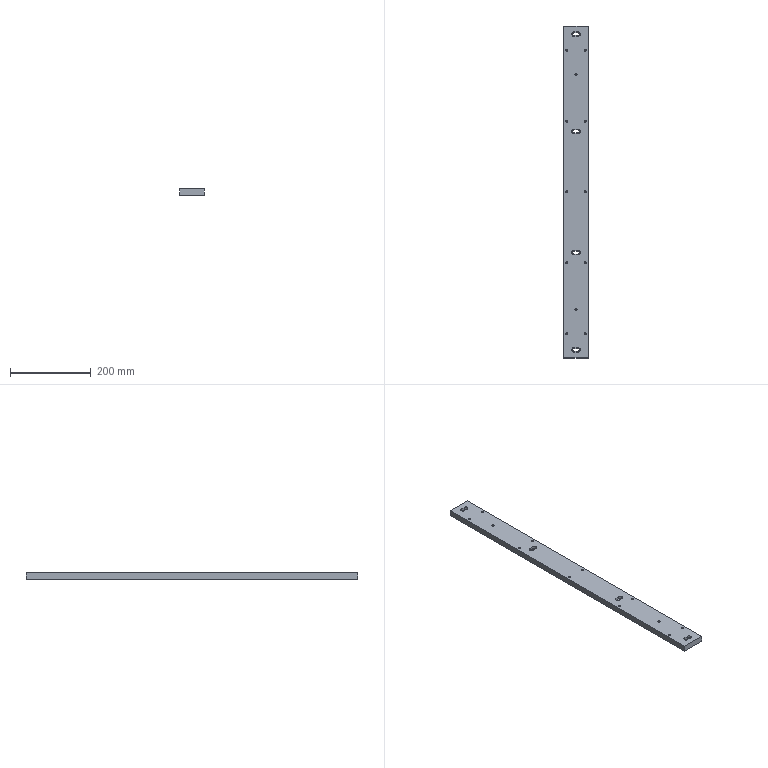Part | SolidWorks | features HoleWzd 3, ICE 2, Extrusion 1, LPattern 1 | 1 solid | 74 faces | box 60 x 820 x 15 mm | volume 725646 mm3 | cylinder 48 | plane 26 | commonest cylinder face diameters 5 x20 6.6 x12 11 x12 5.5 x4